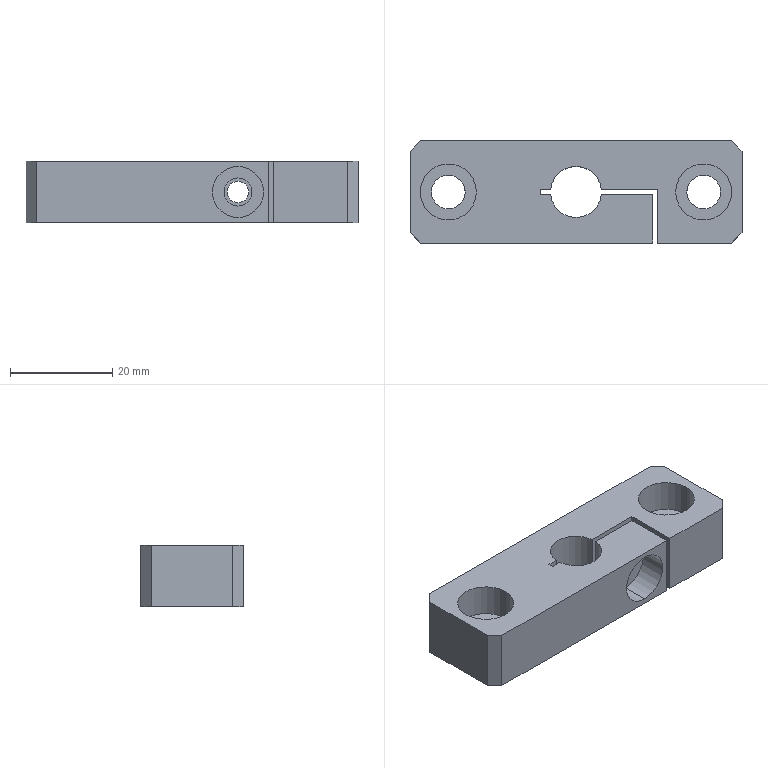Part | SolidWorks | features HoleWzd 3, ICE 2, Chamfer 1, Extrusion 1 | 1 solid | 37 faces | box 65 x 20 x 12 mm | volume 12039 mm3 | plane 21 | cylinder 16 | commonest cylinder face diameters 6.6 x4 10 x4 11 x4 4.2 x2 5.5 x2
STEP:
#1=CARTESIAN_POINT('',(19.5,0.,-0.4));
#2=VERTEX_POINT('',#1);
#3=CARTESIAN_POINT('',(30.5,0.,-0.4));
#4=VERTEX_POINT('',#3);
#5=CARTESIAN_POINT('',(25.,0.,-0.4));
#6=DIRECTION('',(0.,0.,1.));
#7=DIRECTION('',(1.,0.,0.));
#8=AXIS2_PLACEMENT_3D('',#5,#6,#7);
#9=CIRCLE('',#8,5.5);
#10=EDGE_CURVE('',#2,#4,#9,.T.);
#11=ORIENTED_EDGE('',*,*,#10,.F.);
#12=CARTESIAN_POINT('',(19.5,0.,6.));
#13=VERTEX_POINT('',#12);
#14=CARTESIAN_POINT('',(19.5,0.,6.));
#15=DIRECTION('',(0.,0.,1.));
#16=VECTOR('',#15,1000.);
#17=LINE('',#14,#16);
#18=EDGE_CURVE('',#2,#13,#17,.T.);
#19=ORIENTED_EDGE('',*,*,#18,.T.);
#20=CARTESIAN_POINT('',(30.5,0.,6.));
#21=VERTEX_POINT('',#20);
#22=CARTESIAN_POINT('',(25.,0.,6.));
#23=DIRECTION('',(0.,0.,1.));
#24=DIRECTION('',(1.,0.,0.));
#25=AXIS2_PLACEMENT_3D('',#22,#23,#24);
#26=CIRCLE('',#25,5.5);
#27=EDGE_CURVE('',#13,#21,#26,.T.);
#28=ORIENTED_EDGE('',*,*,#27,.T.);
#29=CARTESIAN_POINT('',(30.5,0.,6.));
#30=DIRECTION('',(0.,0.,1.));
#31=VECTOR('',#30,1000.);
#32=LINE('',#29,#31);
#33=EDGE_CURVE('',#4,#21,#32,.T.);
#34=ORIENTED_EDGE('',*,*,#33,.F.);
#35=EDGE_LOOP('',(#11,#19,#28,#34));
#36=FACE_OUTER_BOUND('',#35,.T.);
#37=CARTESIAN_POINT('',(25.,0.,6.));
#38=DIRECTION('',(0.,0.,1.));
#39=DIRECTION('',(1.,0.,0.));
#40=AXIS2_PLACEMENT_3D('',#37,#38,#39);
#41=CYLINDRICAL_SURFACE('',#40,5.5);
#42=ADVANCED_FACE('',(#36),#41,.F.);
#43=CARTESIAN_POINT('',(21.7,0.,-6.));
#44=VERTEX_POINT('',#43);
#45=CARTESIAN_POINT('',(28.3,0.,-6.));
#46=VERTEX_POINT('',#45);
#47=CARTESIAN_POINT('',(25.,0.,-6.));
#48=DIRECTION('',(0.,0.,1.));
#49=DIRECTION('',(1.,0.,0.));
#50=AXIS2_PLACEMENT_3D('',#47,#48,#49);
#51=CIRCLE('',#50,3.3);
#52=EDGE_CURVE('',#44,#46,#51,.T.);
#53=ORIENTED_EDGE('',*,*,#52,.F.);
#54=CARTESIAN_POINT('',(21.7,0.,-0.4));
#55=VERTEX_POINT('',#54);
#56=CARTESIAN_POINT('',(21.7,0.,6.));
#57=DIRECTION('',(0.,0.,1.));
#58=VECTOR('',#57,1000.);
#59=LINE('',#56,#58);
#60=EDGE_CURVE('',#44,#55,#59,.T.);
#61=ORIENTED_EDGE('',*,*,#60,.T.);
#62=CARTESIAN_POINT('',(28.3,0.,-0.4));
#63=VERTEX_POINT('',#62);
#64=CARTESIAN_POINT('',(25.,0.,-0.4));
#65=DIRECTION('',(0.,0.,1.));
#66=DIRECTION('',(1.,0.,0.));
#67=AXIS2_PLACEMENT_3D('',#64,#65,#66);
#68=CIRCLE('',#67,3.3);
#69=EDGE_CURVE('',#55,#63,#68,.T.);
#70=ORIENTED_EDGE('',*,*,#69,.T.);
#71=CARTESIAN_POINT('',(28.3,0.,6.));
#72=DIRECTION('',(0.,0.,1.));
#73=VECTOR('',#72,1000.);
#74=LINE('',#71,#73);
#75=EDGE_CURVE('',#46,#63,#74,.T.);
#76=ORIENTED_EDGE('',*,*,#75,.F.);
#77=EDGE_LOOP('',(#53,#61,#70,#76));
#78=FACE_OUTER_BOUND('',#77,.T.);
#79=CARTESIAN_POINT('',(25.,0.,6.));
#80=DIRECTION('',(0.,0.,1.));
#81=DIRECTION('',(1.,0.,0.));
#82=AXIS2_PLACEMENT_3D('',#79,#80,#81);
#83=CYLINDRICAL_SURFACE('',#82,3.3);
#84=ADVANCED_FACE('',(#78),#83,.F.);
#85=CARTESIAN_POINT('',(-30.5,0.,-0.4));
#86=VERTEX_POINT('',#85);
#87=CARTESIAN_POINT('',(-19.5,0.,-0.4));
#88=VERTEX_POINT('',#87);
#89=CARTESIAN_POINT('',(-25.,0.,-0.4));
#90=DIRECTION('',(0.,0.,1.));
#91=DIRECTION('',(1.,0.,0.));
#92=AXIS2_PLACEMENT_3D('',#89,#90,#91);
#93=CIRCLE('',#92,5.5);
#94=EDGE_CURVE('',#86,#88,#93,.T.);
#95=ORIENTED_EDGE('',*,*,#94,.F.);
#96=CARTESIAN_POINT('',(-30.5,0.,6.));
#97=VERTEX_POINT('',#96);
#98=CARTESIAN_POINT('',(-30.5,0.,6.));
#99=DIRECTION('',(0.,0.,1.));
#100=VECTOR('',#99,1000.);
#101=LINE('',#98,#100);
#102=EDGE_CURVE('',#86,#97,#101,.T.);
#103=ORIENTED_EDGE('',*,*,#102,.T.);
#104=CARTESIAN_POINT('',(-19.5,0.,6.));
#105=VERTEX_POINT('',#104);
#106=CARTESIAN_POINT('',(-25.,0.,6.));
#107=DIRECTION('',(0.,0.,1.));
#108=DIRECTION('',(1.,0.,0.));
#109=AXIS2_PLACEMENT_3D('',#106,#107,#108);
#110=CIRCLE('',#109,5.5);
#111=EDGE_CURVE('',#97,#105,#110,.T.);
#112=ORIENTED_EDGE('',*,*,#111,.T.);
#113=CARTESIAN_POINT('',(-19.5,0.,6.));
#114=DIRECTION('',(0.,0.,1.));
#115=VECTOR('',#114,1000.);
#116=LINE('',#113,#115);
#117=EDGE_CURVE('',#88,#105,#116,.T.);
#118=ORIENTED_EDGE('',*,*,#117,.F.);
#119=EDGE_LOOP('',(#95,#103,#112,#118));
#120=FACE_OUTER_BOUND('',#119,.T.);
#121=CARTESIAN_POINT('',(-25.,0.,6.));
#122=DIRECTION('',(0.,0.,1.));
#123=DIRECTION('',(1.,0.,0.));
#124=AXIS2_PLACEMENT_3D('',#121,#122,#123);
#125=CYLINDRICAL_SURFACE('',#124,5.5);
#126=ADVANCED_FACE('',(#120),#125,.F.);
#127=CARTESIAN_POINT('',(-28.3,0.,-6.));
#128=VERTEX_POINT('',#127);
#129=CARTESIAN_POINT('',(-21.7,0.,-6.));
#130=VERTEX_POINT('',#129);
#131=CARTESIAN_POINT('',(-25.,0.,-6.));
#132=DIRECTION('',(0.,0.,1.));
#133=DIRECTION('',(1.,0.,0.));
#134=AXIS2_PLACEMENT_3D('',#131,#132,#133);
#135=CIRCLE('',#134,3.3);
#136=EDGE_CURVE('',#128,#130,#135,.T.);
#137=ORIENTED_EDGE('',*,*,#136,.F.);
#138=CARTESIAN_POINT('',(-28.3,0.,-0.4));
#139=VERTEX_POINT('',#138);
#140=CARTESIAN_POINT('',(-28.3,0.,6.));
#141=DIRECTION('',(0.,0.,1.));
#142=VECTOR('',#141,1000.);
#143=LINE('',#140,#142);
#144=EDGE_CURVE('',#128,#139,#143,.T.);
#145=ORIENTED_EDGE('',*,*,#144,.T.);
#146=CARTESIAN_POINT('',(-21.7,0.,-0.4));
#147=VERTEX_POINT('',#146);
#148=CARTESIAN_POINT('',(-25.,0.,-0.4));
#149=DIRECTION('',(0.,0.,1.));
#150=DIRECTION('',(1.,0.,0.));
#151=AXIS2_PLACEMENT_3D('',#148,#149,#150);
#152=CIRCLE('',#151,3.3);
#153=EDGE_CURVE('',#139,#147,#152,.T.);
#154=ORIENTED_EDGE('',*,*,#153,.T.);
#155=CARTESIAN_POINT('',(-21.7,0.,6.));
#156=DIRECTION('',(0.,0.,1.));
#157=VECTOR('',#156,1000.);
#158=LINE('',#155,#157);
#159=EDGE_CURVE('',#130,#147,#158,.T.);
#160=ORIENTED_EDGE('',*,*,#159,.F.);
#161=EDGE_LOOP('',(#137,#145,#154,#160));
#162=FACE_OUTER_BOUND('',#161,.T.);
#163=CARTESIAN_POINT('',(-25.,0.,6.));
#164=DIRECTION('',(0.,0.,1.));
#165=DIRECTION('',(1.,0.,0.));
#166=AXIS2_PLACEMENT_3D('',#163,#164,#165);
#167=CYLINDRICAL_SURFACE('',#166,3.3);
#168=ADVANCED_FACE('',(#162),#167,.F.);
#169=CARTESIAN_POINT('',(9.,0.5,2.1));
#170=VERTEX_POINT('',#169);
#171=CARTESIAN_POINT('',(9.,0.5,-2.1));
#172=VERTEX_POINT('',#171);
#173=CARTESIAN_POINT('',(9.,0.5,0.));
#174=DIRECTION('',(0.,-1.,0.));
#175=DIRECTION('',(0.,0.,1.));
#176=AXIS2_PLACEMENT_3D('',#173,#174,#175);
#177=CIRCLE('',#176,2.1);
#178=EDGE_CURVE('',#170,#172,#177,.T.);
#179=ORIENTED_EDGE('',*,*,#178,.T.);
#180=CARTESIAN_POINT('',(9.,10.,-2.1));
#181=VERTEX_POINT('',#180);
#182=CARTESIAN_POINT('',(9.,10.,-2.1));
#183=DIRECTION('',(0.,1.,0.));
#184=VECTOR('',#183,1000.);
#185=LINE('',#182,#184);
#186=EDGE_CURVE('',#172,#181,#185,.T.);
#187=ORIENTED_EDGE('',*,*,#186,.T.);
#188=CARTESIAN_POINT('',(9.,10.,2.1));
#189=VERTEX_POINT('',#188);
#190=CARTESIAN_POINT('',(9.,10.,0.));
#191=DIRECTION('',(0.,1.,0.));
#192=DIRECTION('',(0.,0.,1.));
#193=AXIS2_PLACEMENT_3D('',#190,#191,#192);
#194=CIRCLE('',#193,2.1);
#195=EDGE_CURVE('',#181,#189,#194,.T.);
#196=ORIENTED_EDGE('',*,*,#195,.T.);
#197=CARTESIAN_POINT('',(9.,10.,2.1));
#198=DIRECTION('',(0.,1.,0.));
#199=VECTOR('',#198,1000.);
#200=LINE('',#197,#199);
#201=EDGE_CURVE('',#170,#189,#200,.T.);
#202=ORIENTED_EDGE('',*,*,#201,.F.);
#203=EDGE_LOOP('',(#179,#187,#196,#202));
#204=FACE_OUTER_BOUND('',#203,.T.);
#205=CARTESIAN_POINT('',(9.,10.,0.));
#206=DIRECTION('',(0.,1.,0.));
#207=DIRECTION('',(0.,0.,1.));
#208=AXIS2_PLACEMENT_3D('',#205,#206,#207);
#209=CYLINDRICAL_SURFACE('',#208,2.1);
#210=ADVANCED_FACE('',(#204),#209,.F.);
#211=CARTESIAN_POINT('',(9.,-4.6,5.));
#212=VERTEX_POINT('',#211);
#213=CARTESIAN_POINT('',(9.,-4.6,-5.));
#214=VERTEX_POINT('',#213);
#215=CARTESIAN_POINT('',(9.,-4.6,0.));
#216=DIRECTION('',(0.,-1.,0.));
#217=DIRECTION('',(0.,0.,-1.));
#218=AXIS2_PLACEMENT_3D('',#215,#216,#217);
#219=CIRCLE('',#218,5.);
#220=EDGE_CURVE('',#212,#214,#219,.T.);
#221=ORIENTED_EDGE('',*,*,#220,.F.);
#222=CARTESIAN_POINT('',(9.,-10.,5.));
#223=VERTEX_POINT('',#222);
#224=CARTESIAN_POINT('',(9.,-10.,5.));
#225=DIRECTION('',(0.,-1.,0.));
#226=VECTOR('',#225,1000.);
#227=LINE('',#224,#226);
#228=EDGE_CURVE('',#212,#223,#227,.T.);
#229=ORIENTED_EDGE('',*,*,#228,.T.);
#230=CARTESIAN_POINT('',(9.,-10.,-5.));
#231=VERTEX_POINT('',#230);
#232=CARTESIAN_POINT('',(9.,-10.,0.));
#233=DIRECTION('',(0.,-1.,0.));
#234=DIRECTION('',(0.,0.,-1.));
#235=AXIS2_PLACEMENT_3D('',#232,#233,#234);
#236=CIRCLE('',#235,5.);
#237=EDGE_CURVE('',#223,#231,#236,.T.);
#238=ORIENTED_EDGE('',*,*,#237,.T.);
#239=CARTESIAN_POINT('',(9.,-10.,-5.));
#240=DIRECTION('',(0.,-1.,0.));
#241=VECTOR('',#240,1000.);
#242=LINE('',#239,#241);
#243=EDGE_CURVE('',#214,#231,#242,.T.);
#244=ORIENTED_EDGE('',*,*,#243,.F.);
#245=EDGE_LOOP('',(#221,#229,#238,#244));
#246=FACE_OUTER_BOUND('',#245,.T.);
#247=CARTESIAN_POINT('',(9.,-10.,0.));
#248=DIRECTION('',(0.,-1.,0.));
#249=DIRECTION('',(0.,0.,-1.));
#250=AXIS2_PLACEMENT_3D('',#247,#248,#249);
#251=CYLINDRICAL_SURFACE('',#250,5.);
#252=ADVANCED_FACE('',(#246),#251,.F.);
#253=CARTESIAN_POINT('',(9.,-0.5,-2.75));
#254=VERTEX_POINT('',#253);
#255=CARTESIAN_POINT('',(9.,-0.5,2.75));
#256=VERTEX_POINT('',#255);
#257=CARTESIAN_POINT('',(9.,-0.5,0.));
#258=DIRECTION('',(0.,1.,0.));
#259=DIRECTION('',(1.,0.,0.));
#260=AXIS2_PLACEMENT_3D('',#257,#258,#259);
#261=CIRCLE('',#260,2.75);
#262=EDGE_CURVE('',#254,#256,#261,.T.);
#263=ORIENTED_EDGE('',*,*,#262,.T.);
#264=CARTESIAN_POINT('',(9.,-4.6,2.75));
#265=VERTEX_POINT('',#264);
#266=CARTESIAN_POINT('',(9.,-10.,2.75));
#267=DIRECTION('',(0.,-1.,0.));
#268=VECTOR('',#267,1000.);
#269=LINE('',#266,#268);
#270=EDGE_CURVE('',#256,#265,#269,.T.);
#271=ORIENTED_EDGE('',*,*,#270,.T.);
#272=CARTESIAN_POINT('',(9.,-4.6,-2.75));
#273=VERTEX_POINT('',#272);
#274=CARTESIAN_POINT('',(9.,-4.6,0.));
#275=DIRECTION('',(0.,-1.,0.));
#276=DIRECTION('',(0.,0.,-1.));
#277=AXIS2_PLACEMENT_3D('',#274,#275,#276);
#278=CIRCLE('',#277,2.75);
#279=EDGE_CURVE('',#265,#273,#278,.T.);
#280=ORIENTED_EDGE('',*,*,#279,.T.);
#281=CARTESIAN_POINT('',(9.,-10.,-2.75));
#282=DIRECTION('',(0.,-1.,0.));
#283=VECTOR('',#282,1000.);
#284=LINE('',#281,#283);
#285=EDGE_CURVE('',#254,#273,#284,.T.);
#286=ORIENTED_EDGE('',*,*,#285,.F.);
#287=EDGE_LOOP('',(#263,#271,#280,#286));
#288=FACE_OUTER_BOUND('',#287,.T.);
#289=CARTESIAN_POINT('',(9.,-10.,0.));
#290=DIRECTION('',(0.,-1.,0.));
#291=DIRECTION('',(0.,0.,-1.));
#292=AXIS2_PLACEMENT_3D('',#289,#290,#291);
#293=CYLINDRICAL_SURFACE('',#292,2.75);
#294=ADVANCED_FACE('',(#288),#293,.F.);
#295=CARTESIAN_POINT('',(4.975,0.5,-6.));
#296=VERTEX_POINT('',#295);
#297=CARTESIAN_POINT('',(16.,0.5,-6.));
#298=VERTEX_POINT('',#297);
#299=CARTESIAN_POINT('',(16.,0.5,-6.));
#300=DIRECTION('',(1.,0.,0.));
#301=VECTOR('',#300,1000.);
#302=LINE('',#299,#301);
#303=EDGE_CURVE('',#296,#298,#302,.T.);
#304=ORIENTED_EDGE('',*,*,#303,.T.);
#305=CARTESIAN_POINT('',(16.,0.5,6.));
#306=VERTEX_POINT('',#305);
#307=CARTESIAN_POINT('',(16.,0.5,6.));
#308=DIRECTION('',(0.,0.,-1.));
#309=VECTOR('',#308,1000.);
#310=LINE('',#307,#309);
#311=EDGE_CURVE('',#306,#298,#310,.T.);
#312=ORIENTED_EDGE('',*,*,#311,.F.);
#313=CARTESIAN_POINT('',(4.975,0.5,6.));
#314=VERTEX_POINT('',#313);
#315=CARTESIAN_POINT('',(16.,0.5,6.));
#316=DIRECTION('',(1.,0.,0.));
#317=VECTOR('',#316,1000.);
#318=LINE('',#315,#317);
#319=EDGE_CURVE('',#314,#306,#318,.T.);
#320=ORIENTED_EDGE('',*,*,#319,.F.);
#321=CARTESIAN_POINT('',(4.975,0.5,6.));
#322=DIRECTION('',(0.,0.,1.));
#323=VECTOR('',#322,1000.);
#324=LINE('',#321,#323);
#325=EDGE_CURVE('',#296,#314,#324,.T.);
#326=ORIENTED_EDGE('',*,*,#325,.F.);
#327=EDGE_LOOP('',(#304,#312,#320,#326));
#328=FACE_OUTER_BOUND('',#327,.T.);
#329=ORIENTED_EDGE('',*,*,#178,.F.);
#330=CARTESIAN_POINT('',(9.,0.5,0.));
#331=DIRECTION('',(0.,-1.,0.));
#332=DIRECTION('',(0.,0.,1.));
#333=AXIS2_PLACEMENT_3D('',#330,#331,#332);
#334=CIRCLE('',#333,2.1);
#335=EDGE_CURVE('',#172,#170,#334,.T.);
#336=ORIENTED_EDGE('',*,*,#335,.F.);
#337=EDGE_LOOP('',(#329,#336));
#338=FACE_BOUND('',#337,.T.);
#339=CARTESIAN_POINT('',(16.,0.5,6.));
#340=DIRECTION('',(0.,1.,0.));
#341=DIRECTION('',(0.,0.,1.));
#342=AXIS2_PLACEMENT_3D('',#339,#340,#341);
#343=PLANE('',#342);
#344=ADVANCED_FACE('',(#328,#338),#343,.F.);
#345=CARTESIAN_POINT('',(15.,-0.5,6.));
#346=VERTEX_POINT('',#345);
#347=CARTESIAN_POINT('',(4.975,-0.5,6.));
#348=VERTEX_POINT('',#347);
#349=CARTESIAN_POINT('',(-7.,-0.5,6.));
#350=DIRECTION('',(-1.,0.,0.));
#351=VECTOR('',#350,1000.);
#352=LINE('',#349,#351);
#353=EDGE_CURVE('',#346,#348,#352,.T.);
#354=ORIENTED_EDGE('',*,*,#353,.F.);
#355=CARTESIAN_POINT('',(15.,-0.5,-6.));
#356=VERTEX_POINT('',#355);
#357=CARTESIAN_POINT('',(15.,-0.5,6.));
#358=DIRECTION('',(0.,0.,-1.));
#359=VECTOR('',#358,1000.);
#360=LINE('',#357,#359);
#361=EDGE_CURVE('',#346,#356,#360,.T.);
#362=ORIENTED_EDGE('',*,*,#361,.T.);
#363=CARTESIAN_POINT('',(4.975,-0.5,-6.));
#364=VERTEX_POINT('',#363);
#365=CARTESIAN_POINT('',(-7.,-0.5,-6.));
#366=DIRECTION('',(-1.,0.,0.));
#367=VECTOR('',#366,1000.);
#368=LINE('',#365,#367);
#369=EDGE_CURVE('',#356,#364,#368,.T.);
#370=ORIENTED_EDGE('',*,*,#369,.T.);
#371=CARTESIAN_POINT('',(4.975,-0.5,6.));
#372=DIRECTION('',(0.,0.,-1.));
#373=VECTOR('',#372,1000.);
#374=LINE('',#371,#373);
#375=EDGE_CURVE('',#348,#364,#374,.T.);
#376=ORIENTED_EDGE('',*,*,#375,.F.);
#377=EDGE_LOOP('',(#354,#362,#370,#376));
#378=FACE_OUTER_BOUND('',#377,.T.);
#379=ORIENTED_EDGE('',*,*,#262,.F.);
#380=CARTESIAN_POINT('',(9.,-0.5,0.));
#381=DIRECTION('',(0.,1.,0.));
#382=DIRECTION('',(1.,0.,0.));
#383=AXIS2_PLACEMENT_3D('',#380,#381,#382);
#384=CIRCLE('',#383,2.75);
#385=EDGE_CURVE('',#256,#254,#384,.T.);
#386=ORIENTED_EDGE('',*,*,#385,.F.);
#387=EDGE_LOOP('',(#379,#386));
#388=FACE_BOUND('',#387,.T.);
#389=CARTESIAN_POINT('',(-7.,-0.5,6.));
#390=DIRECTION('',(0.,-1.,0.));
#391=DIRECTION('',(1.,0.,0.));
#392=AXIS2_PLACEMENT_3D('',#389,#390,#391);
#393=PLANE('',#392);
#394=ADVANCED_FACE('',(#378,#388),#393,.F.);
#395=CARTESIAN_POINT('',(16.,-10.,-6.));
#396=VERTEX_POINT('',#395);
#397=CARTESIAN_POINT('',(30.5,-10.,-6.));
#398=VERTEX_POINT('',#397);
#399=CARTESIAN_POINT('',(-32.5,-10.,-6.));
#400=DIRECTION('',(1.,0.,0.));
#401=VECTOR('',#400,1000.);
#402=LINE('',#399,#401);
#403=EDGE_CURVE('',#396,#398,#402,.T.);
#404=ORIENTED_EDGE('',*,*,#403,.T.);
#405=CARTESIAN_POINT('',(30.5,-10.,6.));
#406=VERTEX_POINT('',#405);
#407=CARTESIAN_POINT('',(30.5,-10.,6.));
#408=DIRECTION('',(0.,0.,1.));
#409=VECTOR('',#408,1000.);
#410=LINE('',#407,#409);
#411=EDGE_CURVE('',#398,#406,#410,.T.);
#412=ORIENTED_EDGE('',*,*,#411,.T.);
#413=CARTESIAN_POINT('',(16.,-10.,6.));
#414=VERTEX_POINT('',#413);
#415=CARTESIAN_POINT('',(-32.5,-10.,6.));
#416=DIRECTION('',(1.,0.,0.));
#417=VECTOR('',#416,1000.);
#418=LINE('',#415,#417);
#419=EDGE_CURVE('',#414,#406,#418,.T.);
#420=ORIENTED_EDGE('',*,*,#419,.F.);
#421=CARTESIAN_POINT('',(16.,-10.,6.));
#422=DIRECTION('',(0.,0.,-1.));
#423=VECTOR('',#422,1000.);
#424=LINE('',#421,#423);
#425=EDGE_CURVE('',#414,#396,#424,.T.);
#426=ORIENTED_EDGE('',*,*,#425,.T.);
#427=EDGE_LOOP('',(#404,#412,#420,#426));
#428=FACE_OUTER_BOUND('',#427,.T.);
#429=CARTESIAN_POINT('',(-32.5,-10.,6.));
#430=DIRECTION('',(0.,1.,0.));
#431=DIRECTION('',(0.,0.,1.));
#432=AXIS2_PLACEMENT_3D('',#429,#430,#431);
#433=PLANE('',#432);
#434=ADVANCED_FACE('',(#428),#433,.F.);
#435=CARTESIAN_POINT('',(-4.975,0.5,-6.));
#436=VERTEX_POINT('',#435);
#437=CARTESIAN_POINT('',(0.,0.,-6.));
#438=DIRECTION('',(0.,0.,-1.));
#439=DIRECTION('',(-1.,0.,0.));
#440=AXIS2_PLACEMENT_3D('',#437,#438,#439);
#441=CIRCLE('',#440,5.);
#442=EDGE_CURVE('',#436,#296,#441,.T.);
#443=ORIENTED_EDGE('',*,*,#442,.T.);
#444=ORIENTED_EDGE('',*,*,#325,.T.);
#445=CARTESIAN_POINT('',(-4.975,0.5,6.));
#446=VERTEX_POINT('',#445);
#447=CARTESIAN_POINT('',(0.,0.,6.));
#448=DIRECTION('',(0.,0.,-1.));
#449=DIRECTION('',(-1.,0.,0.));
#450=AXIS2_PLACEMENT_3D('',#447,#448,#449);
#451=CIRCLE('',#450,5.);
#452=EDGE_CURVE('',#446,#314,#451,.T.);
#453=ORIENTED_EDGE('',*,*,#452,.F.);
#454=CARTESIAN_POINT('',(-4.975,0.5,6.));
#455=DIRECTION('',(0.,0.,-1.));
#456=VECTOR('',#455,1000.);
#457=LINE('',#454,#456);
#458=EDGE_CURVE('',#446,#436,#457,.T.);
#459=ORIENTED_EDGE('',*,*,#458,.T.);
#460=EDGE_LOOP('',(#443,#444,#453,#459));
#461=FACE_OUTER_BOUND('',#460,.T.);
#462=CARTESIAN_POINT('',(0.,0.,6.));
#463=DIRECTION('',(0.,0.,-1.));
#464=DIRECTION('',(-1.,0.,0.));
#465=AXIS2_PLACEMENT_3D('',#462,#463,#464);
#466=CYLINDRICAL_SURFACE('',#465,5.);
#467=ADVANCED_FACE('',(#461),#466,.F.);
#468=CARTESIAN_POINT('',(32.5,-8.,6.));
#469=VERTEX_POINT('',#468);
#470=CARTESIAN_POINT('',(32.5,8.,6.));
#471=VERTEX_POINT('',#470);
#472=CARTESIAN_POINT('',(32.5,-10.,6.));
#473=DIRECTION('',(0.,1.,0.));
#474=VECTOR('',#473,1000.);
#475=LINE('',#472,#474);
#476=EDGE_CURVE('',#469,#471,#475,.T.);
#477=ORIENTED_EDGE('',*,*,#476,.F.);
#478=CARTESIAN_POINT('',(32.5,-8.,-6.));
#479=VERTEX_POINT('',#478);
#480=CARTESIAN_POINT('',(32.5,-8.,6.));
#481=DIRECTION('',(0.,0.,-1.));
#482=VECTOR('',#481,1000.);
#483=LINE('',#480,#482);
#484=EDGE_CURVE('',#469,#479,#483,.T.);
#485=ORIENTED_EDGE('',*,*,#484,.T.);
#486=CARTESIAN_POINT('',(32.5,8.,-6.));
#487=VERTEX_POINT('',#486);
#488=CARTESIAN_POINT('',(32.5,-10.,-6.));
#489=DIRECTION('',(0.,1.,0.));
#490=VECTOR('',#489,1000.);
#491=LINE('',#488,#490);
#492=EDGE_CURVE('',#479,#487,#491,.T.);
#493=ORIENTED_EDGE('',*,*,#492,.T.);
#494=CARTESIAN_POINT('',(32.5,8.,6.));
#495=DIRECTION('',(0.,0.,1.));
#496=VECTOR('',#495,1000.);
#497=LINE('',#494,#496);
#498=EDGE_CURVE('',#487,#471,#497,.T.);
#499=ORIENTED_EDGE('',*,*,#498,.T.);
#500=EDGE_LOOP('',(#477,#485,#493,#499));
#501=FACE_OUTER_BOUND('',#500,.T.);
#502=CARTESIAN_POINT('',(32.5,-10.,6.));
#503=DIRECTION('',(-1.,0.,0.));
#504=DIRECTION('',(0.,0.,1.));
#505=AXIS2_PLACEMENT_3D('',#502,#503,#504);
#506=PLANE('',#505);
#507=ADVANCED_FACE('',(#501),#506,.F.);
#508=CARTESIAN_POINT('',(9.,10.,0.));
#509=DIRECTION('',(0.,1.,0.));
#510=DIRECTION('',(0.,0.,1.));
#511=AXIS2_PLACEMENT_3D('',#508,#509,#510);
#512=CIRCLE('',#511,2.1);
#513=EDGE_CURVE('',#189,#181,#512,.T.);
#514=ORIENTED_EDGE('',*,*,#513,.F.);
#515=ORIENTED_EDGE('',*,*,#195,.F.);
#516=EDGE_LOOP('',(#514,#515));
#517=FACE_BOUND('',#516,.T.);
#518=CARTESIAN_POINT('',(30.5,10.,6.));
#519=VERTEX_POINT('',#518);
#520=CARTESIAN_POINT('',(-30.5,10.,6.));
#521=VERTEX_POINT('',#520);
#522=CARTESIAN_POINT('',(-32.5,10.,6.));
#523=DIRECTION('',(-1.,0.,0.));
#524=VECTOR('',#523,1000.);
#525=LINE('',#522,#524);
#526=EDGE_CURVE('',#519,#521,#525,.T.);
#527=ORIENTED_EDGE('',*,*,#526,.F.);
#528=CARTESIAN_POINT('',(30.5,10.,-6.));
#529=VERTEX_POINT('',#528);
#530=CARTESIAN_POINT('',(30.5,10.,6.));
#531=DIRECTION('',(0.,0.,-1.));
#532=VECTOR('',#531,1000.);
#533=LINE('',#530,#532);
#534=EDGE_CURVE('',#519,#529,#533,.T.);
#535=ORIENTED_EDGE('',*,*,#534,.T.);
#536=CARTESIAN_POINT('',(-30.5,10.,-6.));
#537=VERTEX_POINT('',#536);
#538=CARTESIAN_POINT('',(-32.5,10.,-6.));
#539=DIRECTION('',(-1.,0.,0.));
#540=VECTOR('',#539,1000.);
#541=LINE('',#538,#540);
#542=EDGE_CURVE('',#529,#537,#541,.T.);
#543=ORIENTED_EDGE('',*,*,#542,.T.);
#544=CARTESIAN_POINT('',(-30.5,10.,6.));
#545=DIRECTION('',(0.,0.,1.));
#546=VECTOR('',#545,1000.);
#547=LINE('',#544,#546);
#548=EDGE_CURVE('',#537,#521,#547,.T.);
#549=ORIENTED_EDGE('',*,*,#548,.T.);
#550=EDGE_LOOP('',(#527,#535,#543,#549));
#551=FACE_OUTER_BOUND('',#550,.T.);
#552=CARTESIAN_POINT('',(-32.5,10.,6.));
#553=DIRECTION('',(0.,-1.,0.));
#554=DIRECTION('',(0.,0.,-1.));
#555=AXIS2_PLACEMENT_3D('',#552,#553,#554);
#556=PLANE('',#555);
#557=ADVANCED_FACE('',(#517,#551),#556,.F.);
#558=CARTESIAN_POINT('',(-32.5,8.,-6.));
#559=VERTEX_POINT('',#558);
#560=CARTESIAN_POINT('',(-32.5,-8.,-6.));
#561=VERTEX_POINT('',#560);
#562=CARTESIAN_POINT('',(-32.5,-10.,-6.));
#563=DIRECTION('',(0.,-1.,0.));
#564=VECTOR('',#563,1000.);
#565=LINE('',#562,#564);
#566=EDGE_CURVE('',#559,#561,#565,.T.);
#567=ORIENTED_EDGE('',*,*,#566,.T.);
#568=CARTESIAN_POINT('',(-32.5,-8.,6.));
#569=VERTEX_POINT('',#568);
#570=CARTESIAN_POINT('',(-32.5,-8.,6.));
#571=DIRECTION('',(0.,0.,1.));
#572=VECTOR('',#571,1000.);
#573=LINE('',#570,#572);
#574=EDGE_CURVE('',#561,#569,#573,.T.);
#575=ORIENTED_EDGE('',*,*,#574,.T.);
#576=CARTESIAN_POINT('',(-32.5,8.,6.));
#577=VERTEX_POINT('',#576);
#578=CARTESIAN_POINT('',(-32.5,-10.,6.));
#579=DIRECTION('',(0.,-1.,0.));
#580=VECTOR('',#579,1000.);
#581=LINE('',#578,#580);
#582=EDGE_CURVE('',#577,#569,#581,.T.);
#583=ORIENTED_EDGE('',*,*,#582,.F.);
#584=CARTESIAN_POINT('',(-32.5,8.,6.));
#585=DIRECTION('',(0.,0.,-1.));
#586=VECTOR('',#585,1000.);
#587=LINE('',#584,#586);
#588=EDGE_CURVE('',#577,#559,#587,.T.);
#589=ORIENTED_EDGE('',*,*,#588,.T.);
#590=EDGE_LOOP('',(#567,#575,#583,#589));
#591=FACE_OUTER_BOUND('',#590,.T.);
#592=CARTESIAN_POINT('',(-32.5,-10.,6.));
#593=DIRECTION('',(1.,0.,0.));
#594=DIRECTION('',(0.,0.,-1.));
#595=AXIS2_PLACEMENT_3D('',#592,#593,#594);
#596=PLANE('',#595);
#597=ADVANCED_FACE('',(#591),#596,.F.);
#598=CARTESIAN_POINT('',(9.,-10.,0.));
#599=DIRECTION('',(0.,-1.,0.));
#600=DIRECTION('',(0.,0.,-1.));
#601=AXIS2_PLACEMENT_3D('',#598,#599,#600);
#602=CIRCLE('',#601,5.);
#603=EDGE_CURVE('',#231,#223,#602,.T.);
#604=ORIENTED_EDGE('',*,*,#603,.F.);
#605=ORIENTED_EDGE('',*,*,#237,.F.);
#606=EDGE_LOOP('',(#604,#605));
#607=FACE_BOUND('',#606,.T.);
#608=CARTESIAN_POINT('',(-30.5,-10.,6.));
#609=VERTEX_POINT('',#608);
#610=CARTESIAN_POINT('',(15.,-10.,6.));
#611=VERTEX_POINT('',#610);
#612=CARTESIAN_POINT('',(-32.5,-10.,6.));
#613=DIRECTION('',(1.,0.,0.));
#614=VECTOR('',#613,1000.);
#615=LINE('',#612,#614);
#616=EDGE_CURVE('',#609,#611,#615,.T.);
#617=ORIENTED_EDGE('',*,*,#616,.F.);
#618=CARTESIAN_POINT('',(-30.5,-10.,-6.));
#619=VERTEX_POINT('',#618);
#620=CARTESIAN_POINT('',(-30.5,-10.,6.));
#621=DIRECTION('',(0.,0.,-1.));
#622=VECTOR('',#621,1000.);
#623=LINE('',#620,#622);
#624=EDGE_CURVE('',#609,#619,#623,.T.);
#625=ORIENTED_EDGE('',*,*,#624,.T.);
#626=CARTESIAN_POINT('',(15.,-10.,-6.));
#627=VERTEX_POINT('',#626);
#628=CARTESIAN_POINT('',(-32.5,-10.,-6.));
#629=DIRECTION('',(1.,0.,0.));
#630=VECTOR('',#629,1000.);
#631=LINE('',#628,#630);
#632=EDGE_CURVE('',#619,#627,#631,.T.);
#633=ORIENTED_EDGE('',*,*,#632,.T.);
#634=CARTESIAN_POINT('',(15.,-10.,6.));
#635=DIRECTION('',(0.,0.,-1.));
#636=VECTOR('',#635,1000.);
#637=LINE('',#634,#636);
#638=EDGE_CURVE('',#611,#627,#637,.T.);
#639=ORIENTED_EDGE('',*,*,#638,.F.);
#640=EDGE_LOOP('',(#617,#625,#633,#639));
#641=FACE_OUTER_BOUND('',#640,.T.);
#642=CARTESIAN_POINT('',(-32.5,-10.,6.));
#643=DIRECTION('',(0.,1.,0.));
#644=DIRECTION('',(0.,0.,1.));
#645=AXIS2_PLACEMENT_3D('',#642,#643,#644);
#646=PLANE('',#645);
#647=ADVANCED_FACE('',(#607,#641),#646,.F.);
#648=CARTESIAN_POINT('',(25.,0.,6.));
#649=DIRECTION('',(0.,0.,1.));
#650=DIRECTION('',(1.,0.,0.));
#651=AXIS2_PLACEMENT_3D('',#648,#649,#650);
#652=CIRCLE('',#651,5.5);
#653=EDGE_CURVE('',#21,#13,#652,.T.);
#654=ORIENTED_EDGE('',*,*,#653,.F.);
#655=ORIENTED_EDGE('',*,*,#27,.F.);
#656=EDGE_LOOP('',(#654,#655));
#657=FACE_BOUND('',#656,.T.);
#658=CARTESIAN_POINT('',(-25.,0.,6.));
#659=DIRECTION('',(0.,0.,1.));
#660=DIRECTION('',(1.,0.,0.));
#661=AXIS2_PLACEMENT_3D('',#658,#659,#660);
#662=CIRCLE('',#661,5.5);
#663=EDGE_CURVE('',#105,#97,#662,.T.);
#664=ORIENTED_EDGE('',*,*,#663,.F.);
#665=ORIENTED_EDGE('',*,*,#111,.F.);
#666=EDGE_LOOP('',(#664,#665));
#667=FACE_BOUND('',#666,.T.);
#668=ORIENTED_EDGE('',*,*,#419,.T.);
#669=CARTESIAN_POINT('',(32.5,-8.,6.));
#670=DIRECTION('',(0.7071,0.7071,0.));
#671=VECTOR('',#670,1000.);
#672=LINE('',#669,#671);
#673=EDGE_CURVE('',#406,#469,#672,.T.);
#674=ORIENTED_EDGE('',*,*,#673,.T.);
#675=ORIENTED_EDGE('',*,*,#476,.T.);
#676=CARTESIAN_POINT('',(30.5,10.,6.));
#677=DIRECTION('',(-0.7071,0.7071,0.));
#678=VECTOR('',#677,1000.);
#679=LINE('',#676,#678);
#680=EDGE_CURVE('',#471,#519,#679,.T.);
#681=ORIENTED_EDGE('',*,*,#680,.T.);
#682=ORIENTED_EDGE('',*,*,#526,.T.);
#683=CARTESIAN_POINT('',(-32.5,8.,6.));
#684=DIRECTION('',(-0.7071,-0.7071,0.));
#685=VECTOR('',#684,1000.);
#686=LINE('',#683,#685);
#687=EDGE_CURVE('',#521,#577,#686,.T.);
#688=ORIENTED_EDGE('',*,*,#687,.T.);
#689=ORIENTED_EDGE('',*,*,#582,.T.);
#690=CARTESIAN_POINT('',(-30.5,-10.,6.));
#691=DIRECTION('',(0.7071,-0.7071,0.));
#692=VECTOR('',#691,1000.);
#693=LINE('',#690,#692);
#694=EDGE_CURVE('',#569,#609,#693,.T.);
#695=ORIENTED_EDGE('',*,*,#694,.T.);
#696=ORIENTED_EDGE('',*,*,#616,.T.);
#697=CARTESIAN_POINT('',(15.,-0.5,6.));
#698=DIRECTION('',(0.,1.,0.));
#699=VECTOR('',#698,1000.);
#700=LINE('',#697,#699);
#701=EDGE_CURVE('',#611,#346,#700,.T.);
#702=ORIENTED_EDGE('',*,*,#701,.T.);
#703=ORIENTED_EDGE('',*,*,#353,.T.);
#704=CARTESIAN_POINT('',(-4.975,-0.5,6.));
#705=VERTEX_POINT('',#704);
#706=CARTESIAN_POINT('',(0.,0.,6.));
#707=DIRECTION('',(0.,0.,-1.));
#708=DIRECTION('',(-1.,0.,0.));
#709=AXIS2_PLACEMENT_3D('',#706,#707,#708);
#710=CIRCLE('',#709,5.);
#711=EDGE_CURVE('',#348,#705,#710,.T.);
#712=ORIENTED_EDGE('',*,*,#711,.T.);
#713=CARTESIAN_POINT('',(-7.,-0.5,6.));
#714=VERTEX_POINT('',#713);
#715=CARTESIAN_POINT('',(-7.,-0.5,6.));
#716=DIRECTION('',(-1.,0.,0.));
#717=VECTOR('',#716,1000.);
#718=LINE('',#715,#717);
#719=EDGE_CURVE('',#705,#714,#718,.T.);
#720=ORIENTED_EDGE('',*,*,#719,.T.);
#721=CARTESIAN_POINT('',(-7.,0.5,6.));
#722=VERTEX_POINT('',#721);
#723=CARTESIAN_POINT('',(-7.,0.5,6.));
#724=DIRECTION('',(0.,1.,0.));
#725=VECTOR('',#724,1000.);
#726=LINE('',#723,#725);
#727=EDGE_CURVE('',#714,#722,#726,.T.);
#728=ORIENTED_EDGE('',*,*,#727,.T.);
#729=CARTESIAN_POINT('',(16.,0.5,6.));
#730=DIRECTION('',(1.,0.,0.));
#731=VECTOR('',#730,1000.);
#732=LINE('',#729,#731);
#733=EDGE_CURVE('',#722,#446,#732,.T.);
#734=ORIENTED_EDGE('',*,*,#733,.T.);
#735=ORIENTED_EDGE('',*,*,#452,.T.);
#736=ORIENTED_EDGE('',*,*,#319,.T.);
#737=CARTESIAN_POINT('',(16.,-10.,6.));
#738=DIRECTION('',(0.,-1.,0.));
#739=VECTOR('',#738,1000.);
#740=LINE('',#737,#739);
#741=EDGE_CURVE('',#306,#414,#740,.T.);
#742=ORIENTED_EDGE('',*,*,#741,.T.);
#743=EDGE_LOOP('',(#668,#674,#675,#681,#682,#688,#689,#695,#696,#702,#703,#712,#720,#728,#734,#735,#736,#742));
#744=FACE_OUTER_BOUND('',#743,.T.);
#745=CARTESIAN_POINT('',(0.,0.,6.));
#746=DIRECTION('',(0.,0.,-1.));
#747=DIRECTION('',(-1.,0.,0.));
#748=AXIS2_PLACEMENT_3D('',#745,#746,#747);
#749=PLANE('',#748);
#750=ADVANCED_FACE('',(#657,#667,#744),#749,.F.);
#751=CARTESIAN_POINT('',(25.,0.,-6.));
#752=DIRECTION('',(0.,0.,1.));
#753=DIRECTION('',(1.,0.,0.));
#754=AXIS2_PLACEMENT_3D('',#751,#752,#753);
#755=CIRCLE('',#754,3.3);
#756=EDGE_CURVE('',#46,#44,#755,.T.);
#757=ORIENTED_EDGE('',*,*,#756,.T.);
#758=ORIENTED_EDGE('',*,*,#52,.T.);
#759=EDGE_LOOP('',(#757,#758));
#760=FACE_BOUND('',#759,.T.);
#761=CARTESIAN_POINT('',(-25.,0.,-6.));
#762=DIRECTION('',(0.,0.,1.));
#763=DIRECTION('',(1.,0.,0.));
#764=AXIS2_PLACEMENT_3D('',#761,#762,#763);
#765=CIRCLE('',#764,3.3);
#766=EDGE_CURVE('',#130,#128,#765,.T.);
#767=ORIENTED_EDGE('',*,*,#766,.T.);
#768=ORIENTED_EDGE('',*,*,#136,.T.);
#769=EDGE_LOOP('',(#767,#768));
#770=FACE_BOUND('',#769,.T.);
#771=ORIENTED_EDGE('',*,*,#492,.F.);
#772=CARTESIAN_POINT('',(20.25,-20.25,-6.));
#773=DIRECTION('',(-0.7071,-0.7071,0.));
#774=VECTOR('',#773,1000.);
#775=LINE('',#772,#774);
#776=EDGE_CURVE('',#479,#398,#775,.T.);
#777=ORIENTED_EDGE('',*,*,#776,.T.);
#778=ORIENTED_EDGE('',*,*,#403,.F.);
#779=CARTESIAN_POINT('',(16.,-10.,-6.));
#780=DIRECTION('',(0.,-1.,0.));
#781=VECTOR('',#780,1000.);
#782=LINE('',#779,#781);
#783=EDGE_CURVE('',#298,#396,#782,.T.);
#784=ORIENTED_EDGE('',*,*,#783,.F.);
#785=ORIENTED_EDGE('',*,*,#303,.F.);
#786=ORIENTED_EDGE('',*,*,#442,.F.);
#787=CARTESIAN_POINT('',(-7.,0.5,-6.));
#788=VERTEX_POINT('',#787);
#789=CARTESIAN_POINT('',(16.,0.5,-6.));
#790=DIRECTION('',(1.,0.,0.));
#791=VECTOR('',#790,1000.);
#792=LINE('',#789,#791);
#793=EDGE_CURVE('',#788,#436,#792,.T.);
#794=ORIENTED_EDGE('',*,*,#793,.F.);
#795=CARTESIAN_POINT('',(-7.,-0.5,-6.));
#796=VERTEX_POINT('',#795);
#797=CARTESIAN_POINT('',(-7.,0.5,-6.));
#798=DIRECTION('',(0.,1.,0.));
#799=VECTOR('',#798,1000.);
#800=LINE('',#797,#799);
#801=EDGE_CURVE('',#796,#788,#800,.T.);
#802=ORIENTED_EDGE('',*,*,#801,.F.);
#803=CARTESIAN_POINT('',(-4.975,-0.5,-6.));
#804=VERTEX_POINT('',#803);
#805=CARTESIAN_POINT('',(-7.,-0.5,-6.));
#806=DIRECTION('',(-1.,0.,0.));
#807=VECTOR('',#806,1000.);
#808=LINE('',#805,#807);
#809=EDGE_CURVE('',#804,#796,#808,.T.);
#810=ORIENTED_EDGE('',*,*,#809,.F.);
#811=CARTESIAN_POINT('',(0.,0.,-6.));
#812=DIRECTION('',(0.,0.,-1.));
#813=DIRECTION('',(-1.,0.,0.));
#814=AXIS2_PLACEMENT_3D('',#811,#812,#813);
#815=CIRCLE('',#814,5.);
#816=EDGE_CURVE('',#364,#804,#815,.T.);
#817=ORIENTED_EDGE('',*,*,#816,.F.);
#818=ORIENTED_EDGE('',*,*,#369,.F.);
#819=CARTESIAN_POINT('',(15.,-0.5,-6.));
#820=DIRECTION('',(0.,1.,0.));
#821=VECTOR('',#820,1000.);
#822=LINE('',#819,#821);
#823=EDGE_CURVE('',#627,#356,#822,.T.);
#824=ORIENTED_EDGE('',*,*,#823,.F.);
#825=ORIENTED_EDGE('',*,*,#632,.F.);
#826=CARTESIAN_POINT('',(-20.25,-20.25,-6.));
#827=DIRECTION('',(-0.7071,0.7071,0.));
#828=VECTOR('',#827,1000.);
#829=LINE('',#826,#828);
#830=EDGE_CURVE('',#619,#561,#829,.T.);
#831=ORIENTED_EDGE('',*,*,#830,.T.);
#832=ORIENTED_EDGE('',*,*,#566,.F.);
#833=CARTESIAN_POINT('',(-20.25,20.25,-6.));
#834=DIRECTION('',(0.7071,0.7071,0.));
#835=VECTOR('',#834,1000.);
#836=LINE('',#833,#835);
#837=EDGE_CURVE('',#559,#537,#836,.T.);
#838=ORIENTED_EDGE('',*,*,#837,.T.);
#839=ORIENTED_EDGE('',*,*,#542,.F.);
#840=CARTESIAN_POINT('',(20.25,20.25,-6.));
#841=DIRECTION('',(0.7071,-0.7071,0.));
#842=VECTOR('',#841,1000.);
#843=LINE('',#840,#842);
#844=EDGE_CURVE('',#529,#487,#843,.T.);
#845=ORIENTED_EDGE('',*,*,#844,.T.);
#846=EDGE_LOOP('',(#771,#777,#778,#784,#785,#786,#794,#802,#810,#817,#818,#824,#825,#831,#832,#838,#839,#845));
#847=FACE_OUTER_BOUND('',#846,.T.);
#848=CARTESIAN_POINT('',(0.,0.,-6.));
#849=DIRECTION('',(0.,0.,-1.));
#850=DIRECTION('',(-1.,0.,0.));
#851=AXIS2_PLACEMENT_3D('',#848,#849,#850);
#852=PLANE('',#851);
#853=ADVANCED_FACE('',(#760,#770,#847),#852,.T.);
#854=ORIENTED_EDGE('',*,*,#816,.T.);
#855=CARTESIAN_POINT('',(-4.975,-0.5,6.));
#856=DIRECTION('',(0.,0.,1.));
#857=VECTOR('',#856,1000.);
#858=LINE('',#855,#857);
#859=EDGE_CURVE('',#804,#705,#858,.T.);
#860=ORIENTED_EDGE('',*,*,#859,.T.);
#861=ORIENTED_EDGE('',*,*,#711,.F.);
#862=ORIENTED_EDGE('',*,*,#375,.T.);
#863=EDGE_LOOP('',(#854,#860,#861,#862));
#864=FACE_OUTER_BOUND('',#863,.T.);
#865=CARTESIAN_POINT('',(0.,0.,6.));
#866=DIRECTION('',(0.,0.,-1.));
#867=DIRECTION('',(-1.,0.,0.));
#868=AXIS2_PLACEMENT_3D('',#865,#866,#867);
#869=CYLINDRICAL_SURFACE('',#868,5.);
#870=ADVANCED_FACE('',(#864),#869,.F.);
#871=ORIENTED_EDGE('',*,*,#823,.T.);
#872=ORIENTED_EDGE('',*,*,#361,.F.);
#873=ORIENTED_EDGE('',*,*,#701,.F.);
#874=ORIENTED_EDGE('',*,*,#638,.T.);
#875=EDGE_LOOP('',(#871,#872,#873,#874));
#876=FACE_OUTER_BOUND('',#875,.T.);
#877=CARTESIAN_POINT('',(15.,-0.5,6.));
#878=DIRECTION('',(-1.,0.,0.));
#879=DIRECTION('',(0.,0.,1.));
#880=AXIS2_PLACEMENT_3D('',#877,#878,#879);
#881=PLANE('',#880);
#882=ADVANCED_FACE('',(#876),#881,.F.);
#883=ORIENTED_EDGE('',*,*,#733,.F.);
#884=CARTESIAN_POINT('',(-7.,0.5,6.));
#885=DIRECTION('',(0.,0.,-1.));
#886=VECTOR('',#885,1000.);
#887=LINE('',#884,#886);
#888=EDGE_CURVE('',#722,#788,#887,.T.);
#889=ORIENTED_EDGE('',*,*,#888,.T.);
#890=ORIENTED_EDGE('',*,*,#793,.T.);
#891=ORIENTED_EDGE('',*,*,#458,.F.);
#892=EDGE_LOOP('',(#883,#889,#890,#891));
#893=FACE_OUTER_BOUND('',#892,.T.);
#894=CARTESIAN_POINT('',(16.,0.5,6.));
#895=DIRECTION('',(0.,1.,0.));
#896=DIRECTION('',(0.,0.,1.));
#897=AXIS2_PLACEMENT_3D('',#894,#895,#896);
#898=PLANE('',#897);
#899=ADVANCED_FACE('',(#893),#898,.F.);
#900=ORIENTED_EDGE('',*,*,#809,.T.);
#901=CARTESIAN_POINT('',(-7.,-0.5,6.));
#902=DIRECTION('',(0.,0.,-1.));
#903=VECTOR('',#902,1000.);
#904=LINE('',#901,#903);
#905=EDGE_CURVE('',#714,#796,#904,.T.);
#906=ORIENTED_EDGE('',*,*,#905,.F.);
#907=ORIENTED_EDGE('',*,*,#719,.F.);
#908=ORIENTED_EDGE('',*,*,#859,.F.);
#909=EDGE_LOOP('',(#900,#906,#907,#908));
#910=FACE_OUTER_BOUND('',#909,.T.);
#911=CARTESIAN_POINT('',(-7.,-0.5,6.));
#912=DIRECTION('',(0.,-1.,0.));
#913=DIRECTION('',(1.,0.,0.));
#914=AXIS2_PLACEMENT_3D('',#911,#912,#913);
#915=PLANE('',#914);
#916=ADVANCED_FACE('',(#910),#915,.F.);
#917=ORIENTED_EDGE('',*,*,#801,.T.);
#918=ORIENTED_EDGE('',*,*,#888,.F.);
#919=ORIENTED_EDGE('',*,*,#727,.F.);
#920=ORIENTED_EDGE('',*,*,#905,.T.);
#921=EDGE_LOOP('',(#917,#918,#919,#920));
#922=FACE_OUTER_BOUND('',#921,.T.);
#923=CARTESIAN_POINT('',(-7.,0.5,6.));
#924=DIRECTION('',(-1.,0.,0.));
#925=DIRECTION('',(0.,0.,1.));
#926=AXIS2_PLACEMENT_3D('',#923,#924,#925);
#927=PLANE('',#926);
#928=ADVANCED_FACE('',(#922),#927,.F.);
#929=ORIENTED_EDGE('',*,*,#783,.T.);
#930=ORIENTED_EDGE('',*,*,#425,.F.);
#931=ORIENTED_EDGE('',*,*,#741,.F.);
#932=ORIENTED_EDGE('',*,*,#311,.T.);
#933=EDGE_LOOP('',(#929,#930,#931,#932));
#934=FACE_OUTER_BOUND('',#933,.T.);
#935=CARTESIAN_POINT('',(16.,-10.,6.));
#936=DIRECTION('',(1.,0.,0.));
#937=DIRECTION('',(0.,0.,-1.));
#938=AXIS2_PLACEMENT_3D('',#935,#936,#937);
#939=PLANE('',#938);
#940=ADVANCED_FACE('',(#934),#939,.F.);
#941=ORIENTED_EDGE('',*,*,#270,.F.);
#942=ORIENTED_EDGE('',*,*,#385,.T.);
#943=ORIENTED_EDGE('',*,*,#285,.T.);
#944=CARTESIAN_POINT('',(9.,-4.6,0.));
#945=DIRECTION('',(0.,-1.,0.));
#946=DIRECTION('',(0.,0.,-1.));
#947=AXIS2_PLACEMENT_3D('',#944,#945,#946);
#948=CIRCLE('',#947,2.75);
#949=EDGE_CURVE('',#273,#265,#948,.T.);
#950=ORIENTED_EDGE('',*,*,#949,.T.);
#951=EDGE_LOOP('',(#941,#942,#943,#950));
#952=FACE_OUTER_BOUND('',#951,.T.);
#953=CARTESIAN_POINT('',(9.,-10.,0.));
#954=DIRECTION('',(0.,-1.,0.));
#955=DIRECTION('',(0.,0.,-1.));
#956=AXIS2_PLACEMENT_3D('',#953,#954,#955);
#957=CYLINDRICAL_SURFACE('',#956,2.75);
#958=ADVANCED_FACE('',(#952),#957,.F.);
#959=ORIENTED_EDGE('',*,*,#949,.F.);
#960=ORIENTED_EDGE('',*,*,#279,.F.);
#961=EDGE_LOOP('',(#959,#960));
#962=FACE_BOUND('',#961,.T.);
#963=CARTESIAN_POINT('',(9.,-4.6,0.));
#964=DIRECTION('',(0.,-1.,0.));
#965=DIRECTION('',(0.,0.,-1.));
#966=AXIS2_PLACEMENT_3D('',#963,#964,#965);
#967=CIRCLE('',#966,5.);
#968=EDGE_CURVE('',#214,#212,#967,.T.);
#969=ORIENTED_EDGE('',*,*,#968,.T.);
#970=ORIENTED_EDGE('',*,*,#220,.T.);
#971=EDGE_LOOP('',(#969,#970));
#972=FACE_OUTER_BOUND('',#971,.T.);
#973=CARTESIAN_POINT('',(11.75,-4.6,0.));
#974=DIRECTION('',(0.,1.,0.));
#975=DIRECTION('',(0.,0.,1.));
#976=AXIS2_PLACEMENT_3D('',#973,#974,#975);
#977=PLANE('',#976);
#978=ADVANCED_FACE('',(#962,#972),#977,.F.);
#979=ORIENTED_EDGE('',*,*,#228,.F.);
#980=ORIENTED_EDGE('',*,*,#968,.F.);
#981=ORIENTED_EDGE('',*,*,#243,.T.);
#982=ORIENTED_EDGE('',*,*,#603,.T.);
#983=EDGE_LOOP('',(#979,#980,#981,#982));
#984=FACE_OUTER_BOUND('',#983,.T.);
#985=CARTESIAN_POINT('',(9.,-10.,0.));
#986=DIRECTION('',(0.,-1.,0.));
#987=DIRECTION('',(0.,0.,-1.));
#988=AXIS2_PLACEMENT_3D('',#985,#986,#987);
#989=CYLINDRICAL_SURFACE('',#988,5.);
#990=ADVANCED_FACE('',(#984),#989,.F.);
#991=ORIENTED_EDGE('',*,*,#186,.F.);
#992=ORIENTED_EDGE('',*,*,#335,.T.);
#993=ORIENTED_EDGE('',*,*,#201,.T.);
#994=ORIENTED_EDGE('',*,*,#513,.T.);
#995=EDGE_LOOP('',(#991,#992,#993,#994));
#996=FACE_OUTER_BOUND('',#995,.T.);
#997=CARTESIAN_POINT('',(9.,10.,0.));
#998=DIRECTION('',(0.,1.,0.));
#999=DIRECTION('',(0.,0.,1.));
#1000=AXIS2_PLACEMENT_3D('',#997,#998,#999);
#1001=CYLINDRICAL_SURFACE('',#1000,2.1);
#1002=ADVANCED_FACE('',(#996),#1001,.F.);
#1003=ORIENTED_EDGE('',*,*,#144,.F.);
#1004=ORIENTED_EDGE('',*,*,#766,.F.);
#1005=ORIENTED_EDGE('',*,*,#159,.T.);
#1006=CARTESIAN_POINT('',(-25.,0.,-0.4));
#1007=DIRECTION('',(0.,0.,1.));
#1008=DIRECTION('',(1.,0.,0.));
#1009=AXIS2_PLACEMENT_3D('',#1006,#1007,#1008);
#1010=CIRCLE('',#1009,3.3);
#1011=EDGE_CURVE('',#147,#139,#1010,.T.);
#1012=ORIENTED_EDGE('',*,*,#1011,.T.);
#1013=EDGE_LOOP('',(#1003,#1004,#1005,#1012));
#1014=FACE_OUTER_BOUND('',#1013,.T.);
#1015=CARTESIAN_POINT('',(-25.,0.,6.));
#1016=DIRECTION('',(0.,0.,1.));
#1017=DIRECTION('',(1.,0.,0.));
#1018=AXIS2_PLACEMENT_3D('',#1015,#1016,#1017);
#1019=CYLINDRICAL_SURFACE('',#1018,3.3);
#1020=ADVANCED_FACE('',(#1014),#1019,.F.);
#1021=ORIENTED_EDGE('',*,*,#1011,.F.);
#1022=ORIENTED_EDGE('',*,*,#153,.F.);
#1023=EDGE_LOOP('',(#1021,#1022));
#1024=FACE_BOUND('',#1023,.T.);
#1025=CARTESIAN_POINT('',(-25.,0.,-0.4));
#1026=DIRECTION('',(0.,0.,1.));
#1027=DIRECTION('',(1.,0.,0.));
#1028=AXIS2_PLACEMENT_3D('',#1025,#1026,#1027);
#1029=CIRCLE('',#1028,5.5);
#1030=EDGE_CURVE('',#88,#86,#1029,.T.);
#1031=ORIENTED_EDGE('',*,*,#1030,.T.);
#1032=ORIENTED_EDGE('',*,*,#94,.T.);
#1033=EDGE_LOOP('',(#1031,#1032));
#1034=FACE_OUTER_BOUND('',#1033,.T.);
#1035=CARTESIAN_POINT('',(-21.7,0.,-0.4));
#1036=DIRECTION('',(0.,0.,-1.));
#1037=DIRECTION('',(-1.,0.,0.));
#1038=AXIS2_PLACEMENT_3D('',#1035,#1036,#1037);
#1039=PLANE('',#1038);
#1040=ADVANCED_FACE('',(#1024,#1034),#1039,.F.);
#1041=ORIENTED_EDGE('',*,*,#102,.F.);
#1042=ORIENTED_EDGE('',*,*,#1030,.F.);
#1043=ORIENTED_EDGE('',*,*,#117,.T.);
#1044=ORIENTED_EDGE('',*,*,#663,.T.);
#1045=EDGE_LOOP('',(#1041,#1042,#1043,#1044));
#1046=FACE_OUTER_BOUND('',#1045,.T.);
#1047=CARTESIAN_POINT('',(-25.,0.,6.));
#1048=DIRECTION('',(0.,0.,1.));
#1049=DIRECTION('',(1.,0.,0.));
#1050=AXIS2_PLACEMENT_3D('',#1047,#1048,#1049);
#1051=CYLINDRICAL_SURFACE('',#1050,5.5);
#1052=ADVANCED_FACE('',(#1046),#1051,.F.);
#1053=ORIENTED_EDGE('',*,*,#60,.F.);
#1054=ORIENTED_EDGE('',*,*,#756,.F.);
#1055=ORIENTED_EDGE('',*,*,#75,.T.);
#1056=CARTESIAN_POINT('',(25.,0.,-0.4));
#1057=DIRECTION('',(0.,0.,1.));
#1058=DIRECTION('',(1.,0.,0.));
#1059=AXIS2_PLACEMENT_3D('',#1056,#1057,#1058);
#1060=CIRCLE('',#1059,3.3);
#1061=EDGE_CURVE('',#63,#55,#1060,.T.);
#1062=ORIENTED_EDGE('',*,*,#1061,.T.);
#1063=EDGE_LOOP('',(#1053,#1054,#1055,#1062));
#1064=FACE_OUTER_BOUND('',#1063,.T.);
#1065=CARTESIAN_POINT('',(25.,0.,6.));
#1066=DIRECTION('',(0.,0.,1.));
#1067=DIRECTION('',(1.,0.,0.));
#1068=AXIS2_PLACEMENT_3D('',#1065,#1066,#1067);
#1069=CYLINDRICAL_SURFACE('',#1068,3.3);
#1070=ADVANCED_FACE('',(#1064),#1069,.F.);
#1071=ORIENTED_EDGE('',*,*,#1061,.F.);
#1072=ORIENTED_EDGE('',*,*,#69,.F.);
#1073=EDGE_LOOP('',(#1071,#1072));
#1074=FACE_BOUND('',#1073,.T.);
#1075=CARTESIAN_POINT('',(25.,0.,-0.4));
#1076=DIRECTION('',(0.,0.,1.));
#1077=DIRECTION('',(1.,0.,0.));
#1078=AXIS2_PLACEMENT_3D('',#1075,#1076,#1077);
#1079=CIRCLE('',#1078,5.5);
#1080=EDGE_CURVE('',#4,#2,#1079,.T.);
#1081=ORIENTED_EDGE('',*,*,#1080,.T.);
#1082=ORIENTED_EDGE('',*,*,#10,.T.);
#1083=EDGE_LOOP('',(#1081,#1082));
#1084=FACE_OUTER_BOUND('',#1083,.T.);
#1085=CARTESIAN_POINT('',(28.3,0.,-0.4));
#1086=DIRECTION('',(0.,0.,-1.));
#1087=DIRECTION('',(-1.,0.,0.));
#1088=AXIS2_PLACEMENT_3D('',#1085,#1086,#1087);
#1089=PLANE('',#1088);
#1090=ADVANCED_FACE('',(#1074,#1084),#1089,.F.);
#1091=ORIENTED_EDGE('',*,*,#18,.F.);
#1092=ORIENTED_EDGE('',*,*,#1080,.F.);
#1093=ORIENTED_EDGE('',*,*,#33,.T.);
#1094=ORIENTED_EDGE('',*,*,#653,.T.);
#1095=EDGE_LOOP('',(#1091,#1092,#1093,#1094));
#1096=FACE_OUTER_BOUND('',#1095,.T.);
#1097=CARTESIAN_POINT('',(25.,0.,6.));
#1098=DIRECTION('',(0.,0.,1.));
#1099=DIRECTION('',(1.,0.,0.));
#1100=AXIS2_PLACEMENT_3D('',#1097,#1098,#1099);
#1101=CYLINDRICAL_SURFACE('',#1100,5.5);
#1102=ADVANCED_FACE('',(#1096),#1101,.F.);
#1103=ORIENTED_EDGE('',*,*,#673,.F.);
#1104=ORIENTED_EDGE('',*,*,#411,.F.);
#1105=ORIENTED_EDGE('',*,*,#776,.F.);
#1106=ORIENTED_EDGE('',*,*,#484,.F.);
#1107=EDGE_LOOP('',(#1103,#1104,#1105,#1106));
#1108=FACE_OUTER_BOUND('',#1107,.T.);
#1109=CARTESIAN_POINT('',(32.5,-8.,6.));
#1110=DIRECTION('',(-0.7071,0.7071,0.));
#1111=DIRECTION('',(0.,0.,-1.));
#1112=AXIS2_PLACEMENT_3D('',#1109,#1110,#1111);
#1113=PLANE('',#1112);
#1114=ADVANCED_FACE('',(#1108),#1113,.F.);
#1115=ORIENTED_EDGE('',*,*,#694,.F.);
#1116=ORIENTED_EDGE('',*,*,#574,.F.);
#1117=ORIENTED_EDGE('',*,*,#830,.F.);
#1118=ORIENTED_EDGE('',*,*,#624,.F.);
#1119=EDGE_LOOP('',(#1115,#1116,#1117,#1118));
#1120=FACE_OUTER_BOUND('',#1119,.T.);
#1121=CARTESIAN_POINT('',(-30.5,-10.,6.));
#1122=DIRECTION('',(0.7071,0.7071,0.));
#1123=DIRECTION('',(0.,0.,-1.));
#1124=AXIS2_PLACEMENT_3D('',#1121,#1122,#1123);
#1125=PLANE('',#1124);
#1126=ADVANCED_FACE('',(#1120),#1125,.F.);
#1127=ORIENTED_EDGE('',*,*,#680,.F.);
#1128=ORIENTED_EDGE('',*,*,#498,.F.);
#1129=ORIENTED_EDGE('',*,*,#844,.F.);
#1130=ORIENTED_EDGE('',*,*,#534,.F.);
#1131=EDGE_LOOP('',(#1127,#1128,#1129,#1130));
#1132=FACE_OUTER_BOUND('',#1131,.T.);
#1133=CARTESIAN_POINT('',(30.5,10.,6.));
#1134=DIRECTION('',(-0.7071,-0.7071,0.));
#1135=DIRECTION('',(0.,0.,-1.));
#1136=AXIS2_PLACEMENT_3D('',#1133,#1134,#1135);
#1137=PLANE('',#1136);
#1138=ADVANCED_FACE('',(#1132),#1137,.F.);
#1139=ORIENTED_EDGE('',*,*,#687,.F.);
#1140=ORIENTED_EDGE('',*,*,#548,.F.);
#1141=ORIENTED_EDGE('',*,*,#837,.F.);
#1142=ORIENTED_EDGE('',*,*,#588,.F.);
#1143=EDGE_LOOP('',(#1139,#1140,#1141,#1142));
#1144=FACE_OUTER_BOUND('',#1143,.T.);
#1145=CARTESIAN_POINT('',(-32.5,8.,6.));
#1146=DIRECTION('',(0.7071,-0.7071,0.));
#1147=DIRECTION('',(0.,0.,-1.));
#1148=AXIS2_PLACEMENT_3D('',#1145,#1146,#1147);
#1149=PLANE('',#1148);
#1150=ADVANCED_FACE('',(#1144),#1149,.F.);
#1151=CLOSED_SHELL('',(#42,#84,#126,#168,#210,#252,#294,#344,#394,#434,#467,#507,#557,#597,#647,#750,#853,#870,#882,#899,#916,#928,#940,#958,#978,#990,#1002,#1020,#1040,#1052,#1070,#1090,#1102,#1114,#1126,#1138,#1150));
#1152=MANIFOLD_SOLID_BREP('',#1151);
#1153=CARTESIAN_POINT('',(0.,0.,0.));
#1154=DIRECTION('',(0.,0.,1.));
#1155=DIRECTION('',(1.,0.,0.));
#1156=AXIS2_PLACEMENT_3D('',#1153,#1154,#1155);
#1157=(LENGTH_UNIT()NAMED_UNIT(*)SI_UNIT(.MILLI.,.METRE.));
#1158=UNCERTAINTY_MEASURE_WITH_UNIT(LENGTH_MEASURE(0.00001),#1157,'','');
#1159=(NAMED_UNIT(*)PLANE_ANGLE_UNIT()SI_UNIT($,.RADIAN.));
#1160=(NAMED_UNIT(*)SI_UNIT($,.STERADIAN.)SOLID_ANGLE_UNIT());
#1161=(GEOMETRIC_REPRESENTATION_CONTEXT(3)GLOBAL_UNCERTAINTY_ASSIGNED_CONTEXT((#1158))GLOBAL_UNIT_ASSIGNED_CONTEXT((#1157,#1159,#1160))REPRESENTATION_CONTEXT('',''));
#1162=ADVANCED_BREP_SHAPE_REPRESENTATION('',(#1152,#1156),#1161);